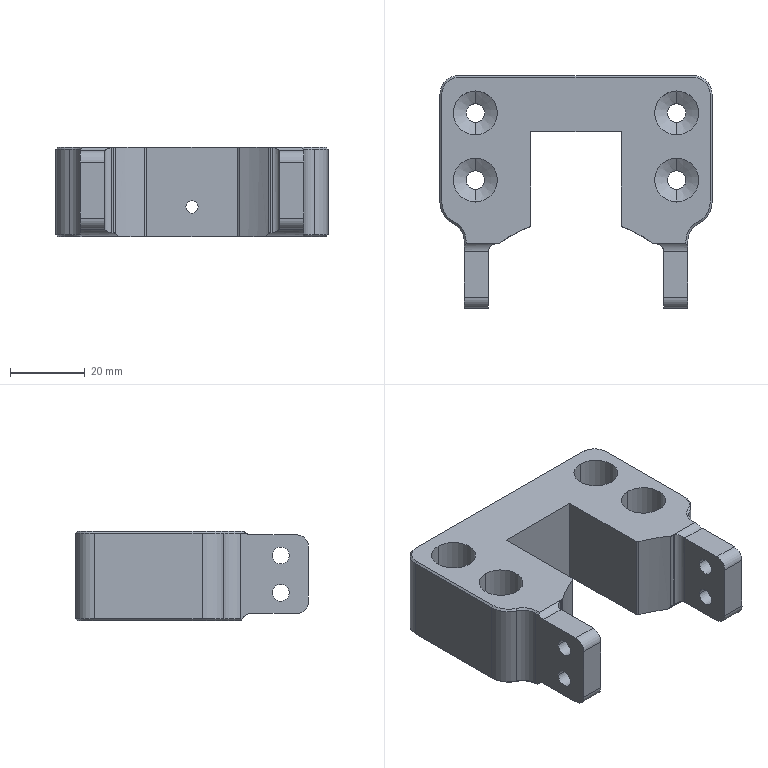NC program | NX | posted with a generic post | part box 73 x 62.4 x 24 mm
Lines 5456 to 6339 of 11507:
(ZLEVEL_PROFILE_COPY_1_COPY_1_COPY_1_1_COPY_COPY_COPY_1 , TOOL : D4)
N10832 T04 M6
N10834 G54
N10836 G17 G0 G90 X22.681 Y-16.85 S7000 M3
N10838 G43 Z30. H4
N10840 Z-0.231
N10842 G94 G1 X22.412 Y-16.271 F800.
N10844 G3 X22.084 Y-16.042 R0.4
N10846 G2 X21.5 Y-15.911 R2.236 F1500.
N10848 G1 X21.119
N10850 G2 X20.882 Y-15.901 R3.
N10852 G3 X20.521 Y-16.073 R0.4
N10854 G1 X20.166 Y-16.589
N10856 G0 X22.595 Y-17.112 Z-0.442
N10858 G1 X22.444 Y-16.527 F800.
N10860 G3 X22.165 Y-16.241 R0.4
N10862 G2 X21.5 Y-15.911 R1.977 F1500.
N10864 G1 X21.119
N10866 G2 X20.66 Y-15.875 R3.
N10868 G3 X20.287 Y-16.02 R0.4
N10870 G1 X19.894 Y-16.508
N10872 G0 X22.489 Y-17.386 Z-0.644
N10874 G1 X22.434 Y-16.785 F800.
N10876 G3 X22.203 Y-16.458 R0.4
N10878 G2 X21.5 Y-15.911 R1.965 F1500.
N10880 G1 X21.119
N10882 G2 X20.494 Y-15.845 R3.
N10884 G3 X20.113 Y-15.968 R0.4
N10886 G1 X19.694 Y-16.433
N10888 G0 X22.362 Y-17.646 Z-0.807
N10890 G1 X22.388 Y-17.042 F800.
N10892 G3 X22.203 Y-16.688 R0.4
N10894 G2 X21.5 Y-15.911 R1.975 F1500.
N10896 G1 X21.119
N10898 G2 X20.335 Y-15.806 R3.
N10900 G3 X19.948 Y-15.909 R0.4
N10902 G1 X19.504 Y-16.35
N10904 G0 X22.15 Y-17.871 Z-0.92
N10906 G1 X22.259 Y-17.277 F800.
N10908 G3 X22.124 Y-16.9 R0.4
N10910 G2 X21.5 Y-15.911 R1.961 F1500.
N10912 G1 X21.119
N10914 G2 X20.184 Y-15.761 R3.
N10916 G3 X19.793 Y-15.843 R0.4
N10918 G1 X19.326 Y-16.261
N10920 G0 X21.945 Y-18.069 Z-0.981
N10922 G1 X22.115 Y-17.491 F800.
N10924 G3 X22.021 Y-17.103 R0.4
N10926 G2 X21.5 Y-15.911 R1.903 F1500.
N10928 G1 X21.119
N10930 G2 X20.038 Y-15.709 R3.
N10932 G3 X19.643 Y-15.771 R0.4
N10934 G1 X19.155 Y-16.164
N10936 G0 X21.761 Y-18.168 Z-1.001
N10938 G1 X21.983 Y-17.59 F800.
N10940 G3 X21.921 Y-17.195 R0.4
N10942 G2 X21.5 Y-15.911 R1.897 F1500.
N10944 G1 X21.119
N10946 G2 X19.957 Y-15.676 R3.
N10948 G3 X19.561 Y-15.727 R0.4
N10950 G1 X19.062 Y-16.106
N10952 G0 X20.7 Y-19.155 Z-1.052
N10954 G1 X21.3 Y-18.808 F800.
N10956 G3 X21.5 Y-18.462 R0.4
N10958 G1 Y-15.911 F1500.
N10960 X21.119
N10962 G2 X19.585 Y-15.489 R3.
N10964 G3 X19.185 Y-15.483 R0.4
N10966 G1 X18.623 Y-15.798
N10968 G0 X20.7 Y-19.155 Z-1.155
N10970 G1 X21.3 Y-18.808 F800.
N10972 G3 X21.5 Y-18.462 R0.4
N10974 G1 Y-15.911 F1500.
N10976 X21.119
N10978 G2 X19.585 Y-15.489 R3.
N10980 G3 X19.185 Y-15.483 R0.4
N10982 G1 X18.623 Y-15.798
N10984 G0 X20.7 Y-19.155 Z-1.309
N10986 G1 X21.3 Y-18.808 F800.
N10988 G3 X21.5 Y-18.462 R0.4
N10990 G1 Y-15.911 F1500.
N10992 X21.119
N10994 G2 X19.585 Y-15.489 R3.
N10996 G3 X19.185 Y-15.483 R0.4
N10998 G1 X18.623 Y-15.798
N11000 G0 X20.7 Y-19.155 Z-1.51
N11002 G1 X21.3 Y-18.808 F800.
N11004 G3 X21.5 Y-18.462 R0.4
N11006 G1 Y-15.911 F1500.
N11008 X21.119
N11010 G2 X19.585 Y-15.489 R3.
N11012 G3 X19.185 Y-15.483 R0.4
N11014 G1 X18.623 Y-15.798
N11016 G0 X20.7 Y-19.155 Z-1.756
N11018 G1 X21.3 Y-18.808 F800.
N11020 G3 X21.5 Y-18.462 R0.4
N11022 G1 Y-15.911 F1500.
N11024 X21.119
N11026 G2 X19.585 Y-15.489 R3.
N11028 G3 X19.185 Y-15.483 R0.4
N11030 G1 X18.623 Y-15.798
N11032 G0 X20.7 Y-19.155 Z-2.041
N11034 G1 X21.3 Y-18.808 F800.
N11036 G3 X21.5 Y-18.462 R0.4
N11038 G1 Y-15.911 F1500.
N11040 X21.119
N11042 G2 X19.585 Y-15.489 R3.
N11044 G3 X19.185 Y-15.483 R0.4
N11046 G1 X18.623 Y-15.798
N11048 G0 X20.7 Y-19.155 Z-2.361
N11050 G1 X21.3 Y-18.808 F800.
N11052 G3 X21.5 Y-18.462 R0.4
N11054 G1 Y-15.911 F1500.
N11056 X21.119
N11058 G2 X19.585 Y-15.489 R3.
N11060 G3 X19.185 Y-15.483 R0.4
N11062 G1 X18.623 Y-15.798
N11064 G0 X20.7 Y-19.155 Z-2.71
N11066 G1 X21.3 Y-18.808 F800.
N11068 G3 X21.5 Y-18.462 R0.4
N11070 G1 Y-15.911 F1500.
N11072 X21.119
N11074 G2 X19.585 Y-15.489 R3.
N11076 G3 X19.185 Y-15.483 R0.4
N11078 G1 X18.623 Y-15.798
N11080 G0 X20.7 Y-19.155 Z-3.082
N11082 G1 X21.3 Y-18.808 F800.
N11084 G3 X21.5 Y-18.462 R0.4
N11086 G1 Y-15.911 F1500.
N11088 X21.119
N11090 G2 X19.585 Y-15.489 R3.
N11092 G3 X19.185 Y-15.483 R0.4
N11094 G1 X18.623 Y-15.798
N11096 G0 X20.7 Y-19.155 Z-3.47
N11098 G1 X21.3 Y-18.808 F800.
N11100 G3 X21.5 Y-18.462 R0.4
N11102 G1 Y-15.911 F1500.
N11104 X21.119
N11106 G2 X19.585 Y-15.489 R3.
N11108 G3 X19.185 Y-15.483 R0.4
N11110 G1 X18.623 Y-15.798
N11112 G0 X20.7 Y-19.155 Z-3.867
N11114 G1 X21.3 Y-18.808 F800.
N11116 G3 X21.5 Y-18.462 R0.4
N11118 G1 Y-15.911 F1500.
N11120 X21.119
N11122 G2 X19.585 Y-15.489 R3.
N11124 G3 X19.185 Y-15.483 R0.4
N11126 G1 X18.623 Y-15.798
N11128 G0 X20.7 Y-19.155 Z-4.267
N11130 G1 X21.3 Y-18.808 F800.
N11132 G3 X21.5 Y-18.462 R0.4
N11134 G1 Y-15.911 F1500.
N11136 X21.119
N11138 G2 X19.585 Y-15.489 R3.
N11140 G3 X19.185 Y-15.483 R0.4
N11142 G1 X18.623 Y-15.798
N11144 G0 X20.7 Y-19.155 Z-4.667
N11146 G1 X21.3 Y-18.808 F800.
N11148 G3 X21.5 Y-18.462 R0.4
N11150 G1 Y-15.911 F1500.
N11152 X21.119
N11154 G2 X19.585 Y-15.489 R3.
N11156 G3 X19.185 Y-15.483 R0.4
N11158 G1 X18.623 Y-15.798
N11160 G0 X20.7 Y-19.155 Z-5.067
N11162 G1 X21.3 Y-18.808 F800.
N11164 G3 X21.5 Y-18.462 R0.4
N11166 G1 Y-15.911 F1500.
N11168 X21.119
N11170 G2 X19.585 Y-15.489 R3.
N11172 G3 X19.185 Y-15.483 R0.4
N11174 G1 X18.623 Y-15.798
N11176 G0 X20.7 Y-19.155 Z-5.467
N11178 G1 X21.3 Y-18.808 F800.
N11180 G3 X21.5 Y-18.462 R0.4
N11182 G1 Y-15.911 F1500.
N11184 X21.119
N11186 G2 X19.585 Y-15.489 R3.
N11188 G3 X19.185 Y-15.483 R0.4
N11190 G1 X18.623 Y-15.798
N11192 G0 X20.7 Y-19.155 Z-5.867
N11194 G1 X21.3 Y-18.808 F800.
N11196 G3 X21.5 Y-18.462 R0.4
N11198 G1 Y-15.911 F1500.
N11200 X21.119
N11202 G2 X19.585 Y-15.489 R3.
N11204 G3 X19.185 Y-15.483 R0.4
N11206 G1 X18.623 Y-15.798
N11208 G0 X20.7 Y-19.155 Z-6.267
N11210 G1 X21.3 Y-18.808 F800.
N11212 G3 X21.5 Y-18.462 R0.4
N11214 G1 Y-15.911 F1500.
N11216 X21.119
N11218 G2 X19.585 Y-15.489 R3.
N11220 G3 X19.185 Y-15.483 R0.4
N11222 G1 X18.623 Y-15.798
N11224 G0 X20.7 Y-19.155 Z-6.667
N11226 G1 X21.3 Y-18.808 F800.
N11228 G3 X21.5 Y-18.462 R0.4
N11230 G1 Y-15.911 F1500.
N11232 X21.119
N11234 G2 X19.585 Y-15.489 R3.
N11236 G3 X19.185 Y-15.483 R0.4
N11238 G1 X18.623 Y-15.798
N11240 G0 X20.7 Y-19.155 Z-7.067
N11242 G1 X21.3 Y-18.808 F800.
N11244 G3 X21.5 Y-18.462 R0.4
N11246 G1 Y-15.911 F1500.
N11248 X21.119
N11250 G2 X19.585 Y-15.489 R3.
N11252 G3 X19.185 Y-15.483 R0.4
N11254 G1 X18.623 Y-15.798
N11256 G0 X20.7 Y-19.155 Z-7.467
N11258 G1 X21.3 Y-18.808 F800.
N11260 G3 X21.5 Y-18.462 R0.4
N11262 G1 Y-15.911 F1500.
N11264 X21.119
N11266 G2 X19.585 Y-15.489 R3.
N11268 G3 X19.185 Y-15.483 R0.4
N11270 G1 X18.623 Y-15.798
N11272 G0 X20.7 Y-19.155 Z-7.867
N11274 G1 X21.3 Y-18.808 F800.
N11276 G3 X21.5 Y-18.462 R0.4
N11278 G1 Y-15.911 F1500.
N11280 X21.119
N11282 G2 X19.585 Y-15.489 R3.
N11284 G3 X19.185 Y-15.483 R0.4
N11286 G1 X18.623 Y-15.798
N11288 G0 X20.7 Y-19.155 Z-8.267
N11290 G1 X21.3 Y-18.808 F800.
N11292 G3 X21.5 Y-18.462 R0.4
N11294 G1 Y-15.911 F1500.
N11296 X21.119
N11298 G2 X19.585 Y-15.489 R3.
N11300 G3 X19.185 Y-15.483 R0.4
N11302 G1 X18.623 Y-15.798
N11304 G0 X20.7 Y-19.155 Z-8.667
N11306 G1 X21.3 Y-18.808 F800.
N11308 G3 X21.5 Y-18.462 R0.4
N11310 G1 Y-15.911 F1500.
N11312 X21.119
N11314 G2 X19.585 Y-15.489 R3.
N11316 G3 X19.185 Y-15.483 R0.4
N11318 G1 X18.623 Y-15.798
N11320 G0 X20.7 Y-19.155 Z-9.067
N11322 G1 X21.3 Y-18.808 F800.
N11324 G3 X21.5 Y-18.462 R0.4
N11326 G1 Y-15.911 F1500.
N11328 X21.119
N11330 G2 X19.585 Y-15.489 R3.
N11332 G3 X19.185 Y-15.483 R0.4
N11334 G1 X18.623 Y-15.798
N11336 G0 X20.7 Y-19.155 Z-9.467
N11338 G1 X21.3 Y-18.808 F800.
N11340 G3 X21.5 Y-18.462 R0.4
N11342 G1 Y-15.911 F1500.
N11344 X21.119
N11346 G2 X19.585 Y-15.489 R3.
N11348 G3 X19.185 Y-15.483 R0.4
N11350 G1 X18.623 Y-15.798
N11352 G0 X20.7 Y-19.155 Z-9.867
N11354 G1 X21.3 Y-18.808 F800.
N11356 G3 X21.5 Y-18.462 R0.4
N11358 G1 Y-15.911 F1500.
N11360 X21.119
N11362 G2 X19.585 Y-15.489 R3.
N11364 G3 X19.185 Y-15.483 R0.4
N11366 G1 X18.623 Y-15.798
N11368 G0 X20.7 Y-19.155 Z-10.267
N11370 G1 X21.3 Y-18.808 F800.
N11372 G3 X21.5 Y-18.462 R0.4
N11374 G1 Y-15.911 F1500.
N11376 X21.119
N11378 G2 X19.585 Y-15.489 R3.
N11380 G3 X19.185 Y-15.483 R0.4
N11382 G1 X18.623 Y-15.798
N11384 G0 X20.7 Y-19.155 Z-10.667
N11386 G1 X21.3 Y-18.808 F800.
N11388 G3 X21.5 Y-18.462 R0.4
N11390 G1 Y-15.911 F1500.
N11392 X21.119
N11394 G2 X19.585 Y-15.489 R3.
N11396 G3 X19.185 Y-15.483 R0.4
N11398 G1 X18.623 Y-15.798
N11400 G0 X20.7 Y-19.155 Z-11.067
N11402 G1 X21.3 Y-18.808 F800.
N11404 G3 X21.5 Y-18.462 R0.4
N11406 G1 Y-15.911 F1500.
N11408 X21.119
N11410 G2 X19.585 Y-15.489 R3.
N11412 G3 X19.185 Y-15.483 R0.4
N11414 G1 X18.623 Y-15.798
N11416 G0 X20.7 Y-19.155 Z-11.467
N11418 G1 X21.3 Y-18.808 F800.
N11420 G3 X21.5 Y-18.462 R0.4
N11422 G1 Y-15.911 F1500.
N11424 X21.119
N11426 G2 X19.585 Y-15.489 R3.
N11428 G3 X19.185 Y-15.483 R0.4
N11430 G1 X18.623 Y-15.798
N11432 G0 X20.7 Y-19.155 Z-11.867
N11434 G1 X21.3 Y-18.808 F800.
N11436 G3 X21.5 Y-18.462 R0.4
N11438 G1 Y-15.911 F1500.
N11440 X21.119
N11442 G2 X19.585 Y-15.489 R3.
N11444 G3 X19.185 Y-15.483 R0.4
N11446 G1 X18.623 Y-15.798
N11448 G0 X20.7 Y-19.155 Z-12.267
N11450 G1 X21.3 Y-18.808 F800.
N11452 G3 X21.5 Y-18.462 R0.4
N11454 G1 Y-15.911 F1500.
N11456 X21.119
N11458 G2 X19.585 Y-15.489 R3.
N11460 G3 X19.185 Y-15.483 R0.4
N11462 G1 X18.623 Y-15.798
N11464 G0 X20.7 Y-19.155 Z-12.667
N11466 G1 X21.3 Y-18.808 F800.
N11468 G3 X21.5 Y-18.462 R0.4
N11470 G1 Y-15.911 F1500.
N11472 X21.119
N11474 G2 X19.585 Y-15.489 R3.
N11476 G3 X19.185 Y-15.483 R0.4
N11478 G1 X18.623 Y-15.798
N11480 G0 X20.7 Y-19.155 Z-13.067
N11482 G1 X21.3 Y-18.808 F800.
N11484 G3 X21.5 Y-18.462 R0.4
N11486 G1 Y-15.911 F1500.
N11488 X21.119
N11490 G2 X19.585 Y-15.489 R3.
N11492 G3 X19.185 Y-15.483 R0.4
N11494 G1 X18.623 Y-15.798
N11496 G0 X20.7 Y-19.155 Z-13.467
N11498 G1 X21.3 Y-18.808 F800.
N11500 G3 X21.5 Y-18.462 R0.4
N11502 G1 Y-15.911 F1500.
N11504 X21.119
N11506 G2 X19.585 Y-15.489 R3.
N11508 G3 X19.185 Y-15.483 R0.4
N11510 G1 X18.623 Y-15.798
N11512 G0 X20.7 Y-19.155 Z-13.867
N11514 G1 X21.3 Y-18.808 F800.
N11516 G3 X21.5 Y-18.462 R0.4
N11518 G1 Y-15.911 F1500.
N11520 X21.119
N11522 G2 X19.585 Y-15.489 R3.
N11524 G3 X19.185 Y-15.483 R0.4
N11526 G1 X18.623 Y-15.798
N11528 G0 X20.7 Y-19.155 Z-14.267
N11530 G1 X21.3 Y-18.808 F800.
N11532 G3 X21.5 Y-18.462 R0.4
N11534 G1 Y-15.911 F1500.
N11536 X21.119
N11538 G2 X19.585 Y-15.489 R3.
N11540 G3 X19.185 Y-15.483 R0.4
N11542 G1 X18.623 Y-15.798
N11544 G0 X20.7 Y-19.155 Z-14.667
N11546 G1 X21.3 Y-18.808 F800.
N11548 G3 X21.5 Y-18.462 R0.4
N11550 G1 Y-15.911 F1500.
N11552 X21.119
N11554 G2 X19.585 Y-15.489 R3.
N11556 G3 X19.185 Y-15.483 R0.4
N11558 G1 X18.623 Y-15.798
N11560 G0 X20.7 Y-19.155 Z-15.067
N11562 G1 X21.3 Y-18.808 F800.
N11564 G3 X21.5 Y-18.462 R0.4
N11566 G1 Y-15.911 F1500.
N11568 X21.119
N11570 G2 X19.585 Y-15.489 R3.
N11572 G3 X19.185 Y-15.483 R0.4
N11574 G1 X18.623 Y-15.798
N11576 G0 X20.7 Y-19.155 Z-15.467
N11578 G1 X21.3 Y-18.808 F800.
N11580 G3 X21.5 Y-18.462 R0.4
N11582 G1 Y-15.911 F1500.
N11584 X21.119
N11586 G2 X19.585 Y-15.489 R3.
N11588 G3 X19.185 Y-15.483 R0.4
N11590 G1 X18.623 Y-15.798
N11592 G0 X20.7 Y-19.155 Z-15.867
N11594 G1 X21.3 Y-18.808 F800.
N11596 G3 X21.5 Y-18.462 R0.4
N11598 G1 Y-15.911 F1500.
N11600 X21.119
N11602 G2 X19.585 Y-15.489 R3.
N11604 G3 X19.185 Y-15.483 R0.4
N11606 G1 X18.623 Y-15.798
N11608 G0 X20.7 Y-19.155 Z-16.267
N11610 G1 X21.3 Y-18.808 F800.
N11612 G3 X21.5 Y-18.462 R0.4
N11614 G1 Y-15.911 F1500.
N11616 X21.119
N11618 G2 X19.585 Y-15.489 R3.
N11620 G3 X19.185 Y-15.483 R0.4
N11622 G1 X18.623 Y-15.798
N11624 G0 X20.7 Y-19.155 Z-16.667
N11626 G1 X21.3 Y-18.808 F800.
N11628 G3 X21.5 Y-18.462 R0.4
N11630 G1 Y-15.911 F1500.
N11632 X21.119
N11634 G2 X19.585 Y-15.489 R3.
N11636 G3 X19.185 Y-15.483 R0.4
N11638 G1 X18.623 Y-15.798
N11640 G0 X20.7 Y-19.155 Z-17.067
N11642 G1 X21.3 Y-18.808 F800.
N11644 G3 X21.5 Y-18.462 R0.4
N11646 G1 Y-15.911 F1500.
N11648 X21.119
N11650 G2 X19.585 Y-15.489 R3.
N11652 G3 X19.185 Y-15.483 R0.4
N11654 G1 X18.623 Y-15.798
N11656 G0 X20.7 Y-19.155 Z-17.467
N11658 G1 X21.3 Y-18.808 F800.
N11660 G3 X21.5 Y-18.462 R0.4
N11662 G1 Y-15.911 F1500.
N11664 X21.119
N11666 G2 X19.585 Y-15.489 R3.
N11668 G3 X19.185 Y-15.483 R0.4
N11670 G1 X18.623 Y-15.798
N11672 G0 X20.7 Y-19.155 Z-17.867
N11674 G1 X21.3 Y-18.808 F800.
N11676 G3 X21.5 Y-18.462 R0.4
N11678 G1 Y-15.911 F1500.
N11680 X21.119
N11682 G2 X19.585 Y-15.489 R3.
N11684 G3 X19.185 Y-15.483 R0.4
N11686 G1 X18.623 Y-15.798
N11688 G0 X20.7 Y-19.155 Z-18.267
N11690 G1 X21.3 Y-18.808 F800.
N11692 G3 X21.5 Y-18.462 R0.4
N11694 G1 Y-15.911 F1500.
N11696 X21.119
N11698 G2 X19.585 Y-15.489 R3.
N11700 G3 X19.185 Y-15.483 R0.4
N11702 G1 X18.623 Y-15.798
N11704 G0 X20.7 Y-19.155 Z-18.667
N11706 G1 X21.3 Y-18.808 F800.
N11708 G3 X21.5 Y-18.462 R0.4
N11710 G1 Y-15.911 F1500.
N11712 X21.119
N11714 G2 X19.585 Y-15.489 R3.
N11716 G3 X19.185 Y-15.483 R0.4
N11718 G1 X18.623 Y-15.798
N11720 G0 X20.7 Y-19.155 Z-19.067
N11722 G1 X21.3 Y-18.808 F800.
N11724 G3 X21.5 Y-18.462 R0.4
N11726 G1 Y-15.911 F1500.
N11728 X21.119
N11730 G2 X19.585 Y-15.489 R3.
N11732 G3 X19.185 Y-15.483 R0.4
N11734 G1 X18.623 Y-15.798
N11736 G0 X20.7 Y-19.155 Z-19.467
N11738 G1 X21.3 Y-18.808 F800.
N11740 G3 X21.5 Y-18.462 R0.4
N11742 G1 Y-15.911 F1500.
N11744 X21.119
N11746 G2 X19.585 Y-15.489 R3.
N11748 G3 X19.185 Y-15.483 R0.4
N11750 G1 X18.623 Y-15.798
N11752 G0 X20.7 Y-19.155 Z-19.867
N11754 G1 X21.3 Y-18.808 F800.
N11756 G3 X21.5 Y-18.462 R0.4
N11758 G1 Y-15.911 F1500.
N11760 X21.119
N11762 G2 X19.585 Y-15.489 R3.
N11764 G3 X19.185 Y-15.483 R0.4
N11766 G1 X18.623 Y-15.798
N11768 G0 X20.7 Y-19.155 Z-20.267
N11770 G1 X21.3 Y-18.808 F800.
N11772 G3 X21.5 Y-18.462 R0.4
N11774 G1 Y-15.911 F1500.
N11776 X21.119
N11778 G2 X19.585 Y-15.489 R3.
N11780 G3 X19.185 Y-15.483 R0.4
N11782 G1 X18.623 Y-15.798
N11784 G0 X20.7 Y-19.155 Z-20.667
N11786 G1 X21.3 Y-18.808 F800.
N11788 G3 X21.5 Y-18.462 R0.4
N11790 G1 Y-15.911 F1500.
N11792 X21.119
N11794 G2 X19.585 Y-15.489 R3.
N11796 G3 X19.185 Y-15.483 R0.4
N11798 G1 X18.623 Y-15.798
N11800 G0 X20.7 Y-19.155 Z-21.067
N11802 G1 X21.3 Y-18.808 F800.
N11804 G3 X21.5 Y-18.462 R0.4
N11806 G1 Y-15.911 F1500.
N11808 X21.119
N11810 G2 X19.585 Y-15.489 R3.
N11812 G3 X19.185 Y-15.483 R0.4
N11814 G1 X18.623 Y-15.798
N11816 G0 X20.7 Y-19.155 Z-21.467
N11818 G1 X21.3 Y-18.808 F800.
N11820 G3 X21.5 Y-18.462 R0.4
N11822 G1 Y-15.911 F1500.
N11824 X21.119
N11826 G2 X19.585 Y-15.489 R3.
N11828 G3 X19.185 Y-15.483 R0.4
N11830 G1 X18.623 Y-15.798
N11832 G0 X20.7 Y-19.155 Z-21.867
N11834 G1 X21.3 Y-18.808 F800.
N11836 G3 X21.5 Y-18.462 R0.4
N11838 G1 Y-15.911 F1500.
N11840 X21.119
N11842 G2 X19.585 Y-15.489 R3.
N11844 G3 X19.185 Y-15.483 R0.4
N11846 G1 X18.623 Y-15.798
N11848 G0 X20.7 Y-19.155 Z-22.267
N11850 G1 X21.3 Y-18.808 F800.
N11852 G3 X21.5 Y-18.462 R0.4
N11854 G1 Y-15.911 F1500.
N11856 X21.119
N11858 G2 X19.585 Y-15.489 R3.
N11860 G3 X19.185 Y-15.483 R0.4
N11862 G1 X18.623 Y-15.798
N11864 G0 X20.7 Y-19.155 Z-22.667
N11866 G1 X21.3 Y-18.808 F800.
N11868 G3 X21.5 Y-18.462 R0.4
N11870 G1 Y-15.911 F1500.
N11872 X21.119
N11874 G2 X19.585 Y-15.489 R3.
N11876 G3 X19.185 Y-15.483 R0.4
N11878 G1 X18.623 Y-15.798
N11880 G0 X20.7 Y-19.155 Z-23.
N11882 G1 X21.3 Y-18.808 F800.
N11884 G3 X21.5 Y-18.462 R0.4
N11886 G1 Y-15.911 F1500.
N11888 X21.119
N11890 G2 X19.585 Y-15.489 R3.
N11892 G3 X19.185 Y-15.483 R0.4
N11894 G1 X18.623 Y-15.798
N11896 G0 X20.7 Y-19.141 Z-23.334
N11898 G1 X21.3 Y-18.795 F800.
N11900 G3 X21.5 Y-18.449 R0.4
N11902 G1 Y-15.911 F1500.
N11904 X21.119
N11906 G2 X19.599 Y-15.497 R3.
N11908 G3 X19.199 Y-15.494 R0.4
N11910 G1 X18.641 Y-15.81
N11912 G0 X20.7 Y-19.141 Z-23.667
N11914 G1 X21.3 Y-18.795 F800.
N11916 G3 X21.5 Y-18.449 R0.4
N11918 G1 Y-15.911 F1500.
N11920 X21.119
N11922 G2 X19.599 Y-15.497 R3.
N11924 G3 X19.199 Y-15.494 R0.4
N11926 G1 X18.641 Y-15.81
N11928 G0 X20.7 Y-19.141 Z-24.
N11930 G1 X21.3 Y-18.795 F800.
N11932 G3 X21.5 Y-18.449 R0.4
N11934 G1 Y-15.911 F1500.
N11936 X21.119
N11938 G2 X19.599 Y-15.497 R3.
N11940 G3 X19.199 Y-15.494 R0.4
N11942 G1 X18.641 Y-15.81
N11944 G0 Z30.
N11946 X9.3 Y10.354
N11948 Z-0.231
N11950 G1 X9.9 Y10.701 F800.
N11952 G3 X10.1 Y11.047 R0.4
N11954 G1 Y14.2 F1500.
N11956 X6.947
N11958 G3 X6.601 Y14. R0.4
N11960 G1 X6.254 Y13.4
N11962 G0 X9.3 Y10.354 Z-0.442
N11964 G1 X9.9 Y10.701 F800.
N11966 G3 X10.1 Y11.047 R0.4
N11968 G1 Y14.2 F1500.
N11970 X6.947
N11972 G3 X6.601 Y14. R0.4
N11974 G1 X6.254 Y13.4
N11976 G0 X9.3 Y10.354 Z-0.644
N11978 G1 X9.9 Y10.701 F800.
N11980 G3 X10.1 Y11.047 R0.4
N11982 G1 Y14.2 F1500.
N11984 X6.947
N11986 G3 X6.601 Y14. R0.4
N11988 G1 X6.254 Y13.4
N11990 G0 X9.3 Y10.354 Z-0.807
N11992 G1 X9.9 Y10.701 F800.
N11994 G3 X10.1 Y11.047 R0.4
N11996 G1 Y14.2 F1500.
N11998 X6.947
N12000 G3 X6.601 Y14. R0.4
N12002 G1 X6.254 Y13.4
N12004 G0 X9.3 Y10.354 Z-0.92
N12006 G1 X9.9 Y10.701 F800.
N12008 G3 X10.1 Y11.047 R0.4
N12010 G1 Y14.2 F1500.
N12012 X6.947
N12014 G3 X6.601 Y14. R0.4
N12016 G1 X6.254 Y13.4
N12018 G0 X9.3 Y10.354 Z-0.981
N12020 G1 X9.9 Y10.701 F800.
N12022 G3 X10.1 Y11.047 R0.4
N12024 G1 Y14.2 F1500.
N12026 X6.947
N12028 G3 X6.601 Y14. R0.4
N12030 G1 X6.254 Y13.4
N12032 G0 X9.3 Y10.354 Z-1.001
N12034 G1 X9.9 Y10.701 F800.
N12036 G3 X10.1 Y11.047 R0.4
N12038 G1 Y14.2 F1500.
N12040 X6.947
N12042 G3 X6.601 Y14. R0.4
N12044 G1 X6.254 Y13.4
N12046 G0 X9.3 Y10.354 Z-1.052
N12048 G1 X9.9 Y10.701 F800.
N12050 G3 X10.1 Y11.047 R0.4
N12052 G1 Y14.2 F1500.
N12054 X6.947
N12056 G3 X6.601 Y14. R0.4
N12058 G1 X6.254 Y13.4
N12060 G0 X9.3 Y10.354 Z-1.155
N12062 G1 X9.9 Y10.701 F800.
N12064 G3 X10.1 Y11.047 R0.4
N12066 G1 Y14.2 F1500.
N12068 X6.947
N12070 G3 X6.601 Y14. R0.4
N12072 G1 X6.254 Y13.4
N12074 G0 X9.3 Y10.354 Z-1.309
N12076 G1 X9.9 Y10.701 F800.
N12078 G3 X10.1 Y11.047 R0.4
N12080 G1 Y14.2 F1500.
N12082 X6.947
N12084 G3 X6.601 Y14. R0.4
N12086 G1 X6.254 Y13.4
N12088 G0 X9.3 Y10.354 Z-1.51
N12090 G1 X9.9 Y10.701 F800.
N12092 G3 X10.1 Y11.047 R0.4
N12094 G1 Y14.2 F1500.
N12096 X6.947
N12098 G3 X6.601 Y14. R0.4
N12100 G1 X6.254 Y13.4
N12102 G0 X9.3 Y10.354 Z-1.756
N12104 G1 X9.9 Y10.701 F800.
N12106 G3 X10.1 Y11.047 R0.4
N12108 G1 Y14.2 F1500.
N12110 X6.947
N12112 G3 X6.601 Y14. R0.4
N12114 G1 X6.254 Y13.4
N12116 G0 X9.3 Y10.354 Z-2.041
N12118 G1 X9.9 Y10.701 F800.
N12120 G3 X10.1 Y11.047 R0.4
N12122 G1 Y14.2 F1500.
N12124 X6.947
N12126 G3 X6.601 Y14. R0.4
N12128 G1 X6.254 Y13.4
N12130 G0 X9.3 Y10.354 Z-2.361
N12132 G1 X9.9 Y10.701 F800.
N12134 G3 X10.1 Y11.047 R0.4
N12136 G1 Y14.2 F1500.
N12138 X6.947
N12140 G3 X6.601 Y14. R0.4
N12142 G1 X6.254 Y13.4
N12144 G0 X9.3 Y10.354 Z-2.71
N12146 G1 X9.9 Y10.701 F800.
N12148 G3 X10.1 Y11.047 R0.4
N12150 G1 Y14.2 F1500.
N12152 X6.947
N12154 G3 X6.601 Y14. R0.4
N12156 G1 X6.254 Y13.4
N12158 G0 X9.3 Y10.354 Z-3.082
N12160 G1 X9.9 Y10.701 F800.
N12162 G3 X10.1 Y11.047 R0.4
N12164 G1 Y14.2 F1500.
N12166 X6.947
N12168 G3 X6.601 Y14. R0.4
N12170 G1 X6.254 Y13.4
N12172 G0 X9.3 Y10.354 Z-3.47
N12174 G1 X9.9 Y10.701 F800.
N12176 G3 X10.1 Y11.047 R0.4
N12178 G1 Y14.2 F1500.
N12180 X6.947
N12182 G3 X6.601 Y14. R0.4
N12184 G1 X6.254 Y13.4
N12186 G0 X9.3 Y10.354 Z-3.867
N12188 G1 X9.9 Y10.701 F800.
N12190 G3 X10.1 Y11.047 R0.4
N12192 G1 Y14.2 F1500.
N12194 X6.947
N12196 G3 X6.601 Y14. R0.4
N12198 G1 X6.254 Y13.4
N12200 G0 X9.3 Y10.354 Z-4.267
N12202 G1 X9.9 Y10.701 F800.
N12204 G3 X10.1 Y11.047 R0.4
N12206 G1 Y14.2 F1500.
N12208 X6.947
N12210 G3 X6.601 Y14. R0.4
N12212 G1 X6.254 Y13.4
N12214 G0 X9.3 Y10.354 Z-4.667
N12216 G1 X9.9 Y10.701 F800.
N12218 G3 X10.1 Y11.047 R0.4
N12220 G1 Y14.2 F1500.
N12222 X6.947
N12224 G3 X6.601 Y14. R0.4
N12226 G1 X6.254 Y13.4
N12228 G0 X9.3 Y10.354 Z-5.067
N12230 G1 X9.9 Y10.701 F800.
N12232 G3 X10.1 Y11.047 R0.4
N12234 G1 Y14.2 F1500.
N12236 X6.947
N12238 G3 X6.601 Y14. R0.4
N12240 G1 X6.254 Y13.4
N12242 G0 X9.3 Y10.354 Z-5.467
N12244 G1 X9.9 Y10.701 F800.
N12246 G3 X10.1 Y11.047 R0.4
N12248 G1 Y14.2 F1500.
N12250 X6.947
N12252 G3 X6.601 Y14. R0.4
N12254 G1 X6.254 Y13.4
N12256 G0 X9.3 Y10.354 Z-5.867
N12258 G1 X9.9 Y10.701 F800.
N12260 G3 X10.1 Y11.047 R0.4
N12262 G1 Y14.2 F1500.
N12264 X6.947
N12266 G3 X6.601 Y14. R0.4
N12268 G1 X6.254 Y13.4
N12270 G0 X9.3 Y10.354 Z-6.267
N12272 G1 X9.9 Y10.701 F800.
N12274 G3 X10.1 Y11.047 R0.4
N12276 G1 Y14.2 F1500.
N12278 X6.947
N12280 G3 X6.601 Y14. R0.4
N12282 G1 X6.254 Y13.4
N12284 G0 X9.3 Y10.354 Z-6.667
N12286 G1 X9.9 Y10.701 F800.
N12288 G3 X10.1 Y11.047 R0.4
N12290 G1 Y14.2 F1500.
N12292 X6.947
N12294 G3 X6.601 Y14. R0.4
N12296 G1 X6.254 Y13.4
N12298 G0 X9.3 Y10.354 Z-7.067
N12300 G1 X9.9 Y10.701 F800.
N12302 G3 X10.1 Y11.047 R0.4
N12304 G1 Y14.2 F1500.
N12306 X6.947
N12308 G3 X6.601 Y14. R0.4
N12310 G1 X6.254 Y13.4
N12312 G0 X9.3 Y10.354 Z-7.467
N12314 G1 X9.9 Y10.701 F800.
N12316 G3 X10.1 Y11.047 R0.4
N12318 G1 Y14.2 F1500.
N12320 X6.947
N12322 G3 X6.601 Y14. R0.4
N12324 G1 X6.254 Y13.4
N12326 G0 X9.3 Y10.354 Z-7.867
N12328 G1 X9.9 Y10.701 F800.
N12330 G3 X10.1 Y11.047 R0.4
N12332 G1 Y14.2 F1500.
N12334 X6.947
N12336 G3 X6.601 Y14. R0.4
N12338 G1 X6.254 Y13.4
N12340 G0 X9.3 Y10.354 Z-8.267
N12342 G1 X9.9 Y10.701 F800.
N12344 G3 X10.1 Y11.047 R0.4
N12346 G1 Y14.2 F1500.
N12348 X6.947
N12350 G3 X6.601 Y14. R0.4
N12352 G1 X6.254 Y13.4
N12354 G0 X9.3 Y10.354 Z-8.667
N12356 G1 X9.9 Y10.701 F800.
N12358 G3 X10.1 Y11.047 R0.4
N12360 G1 Y14.2 F1500.
N12362 X6.947
N12364 G3 X6.601 Y14. R0.4
N12366 G1 X6.254 Y13.4
N12368 G0 X9.3 Y10.354 Z-9.067
N12370 G1 X9.9 Y10.701 F800.
N12372 G3 X10.1 Y11.047 R0.4
N12374 G1 Y14.2 F1500.
N12376 X6.947
N12378 G3 X6.601 Y14. R0.4
N12380 G1 X6.254 Y13.4
N12382 G0 X9.3 Y10.354 Z-9.467
N12384 G1 X9.9 Y10.701 F800.
N12386 G3 X10.1 Y11.047 R0.4
N12388 G1 Y14.2 F1500.
N12390 X6.947
N12392 G3 X6.601 Y14. R0.4
N12394 G1 X6.254 Y13.4
N12396 G0 X9.3 Y10.354 Z-9.867
N12398 G1 X9.9 Y10.701 F800.
N12400 G3 X10.1 Y11.047 R0.4
N12402 G1 Y14.2 F1500.
N12404 X6.947
N12406 G3 X6.601 Y14. R0.4
N12408 G1 X6.254 Y13.4
N12410 G0 X9.3 Y10.354 Z-10.267
N12412 G1 X9.9 Y10.701 F800.
N12414 G3 X10.1 Y11.047 R0.4
N12416 G1 Y14.2 F1500.
N12418 X6.947
N12420 G3 X6.601 Y14. R0.4
N12422 G1 X6.254 Y13.4
N12424 G0 X9.3 Y10.354 Z-10.667
N12426 G1 X9.9 Y10.701 F800.
N12428 G3 X10.1 Y11.047 R0.4
N12430 G1 Y14.2 F1500.
N12432 X6.947
N12434 G3 X6.601 Y14. R0.4
N12436 G1 X6.254 Y13.4
N12438 G0 X9.3 Y10.354 Z-11.067
N12440 G1 X9.9 Y10.701 F800.
N12442 G3 X10.1 Y11.047 R0.4
N12444 G1 Y14.2 F1500.
N12446 X6.947
N12448 G3 X6.601 Y14. R0.4
N12450 G1 X6.254 Y13.4
N12452 G0 X9.3 Y10.354 Z-11.467
N12454 G1 X9.9 Y10.701 F800.
N12456 G3 X10.1 Y11.047 R0.4
N12458 G1 Y14.2 F1500.
N12460 X6.947
N12462 G3 X6.601 Y14. R0.4
N12464 G1 X6.254 Y13.4
N12466 G0 X9.3 Y10.354 Z-11.867
N12468 G1 X9.9 Y10.701 F800.
N12470 G3 X10.1 Y11.047 R0.4
N12472 G1 Y14.2 F1500.
N12474 X6.947
N12476 G3 X6.601 Y14. R0.4
N12478 G1 X6.254 Y13.4
N12480 G0 X9.3 Y10.354 Z-12.267
N12482 G1 X9.9 Y10.701 F800.
N12484 G3 X10.1 Y11.047 R0.4
N12486 G1 Y14.2 F1500.
N12488 X6.947
N12490 G3 X6.601 Y14. R0.4
N12492 G1 X6.254 Y13.4
N12494 G0 X9.3 Y10.354 Z-12.667
N12496 G1 X9.9 Y10.701 F800.
N12498 G3 X10.1 Y11.047 R0.4
N12500 G1 Y14.2 F1500.
N12502 X6.947
N12504 G3 X6.601 Y14. R0.4
N12506 G1 X6.254 Y13.4
N12508 G0 X9.3 Y10.354 Z-13.067
N12510 G1 X9.9 Y10.701 F800.
N12512 G3 X10.1 Y11.047 R0.4
N12514 G1 Y14.2 F1500.
N12516 X6.947
N12518 G3 X6.601 Y14. R0.4
N12520 G1 X6.254 Y13.4
N12522 G0 X9.3 Y10.354 Z-13.467
N12524 G1 X9.9 Y10.701 F800.
N12526 G3 X10.1 Y11.047 R0.4
N12528 G1 Y14.2 F1500.
N12530 X6.947
N12532 G3 X6.601 Y14. R0.4
N12534 G1 X6.254 Y13.4
N12536 G0 X9.3 Y10.354 Z-13.867
N12538 G1 X9.9 Y10.701 F800.
N12540 G3 X10.1 Y11.047 R0.4
N12542 G1 Y14.2 F1500.
N12544 X6.947
N12546 G3 X6.601 Y14. R0.4
N12548 G1 X6.254 Y13.4
N12550 G0 X9.3 Y10.354 Z-14.267
N12552 G1 X9.9 Y10.701 F800.
N12554 G3 X10.1 Y11.047 R0.4
N12556 G1 Y14.2 F1500.
N12558 X6.947
N12560 G3 X6.601 Y14. R0.4
N12562 G1 X6.254 Y13.4
N12564 G0 X9.3 Y10.354 Z-14.667
N12566 G1 X9.9 Y10.701 F800.
N12568 G3 X10.1 Y11.047 R0.4
N12570 G1 Y14.2 F1500.
N12572 X6.947
N12574 G3 X6.601 Y14. R0.4
N12576 G1 X6.254 Y13.4
N12578 G0 X9.3 Y10.354 Z-15.067
N12580 G1 X9.9 Y10.701 F800.
N12582 G3 X10.1 Y11.047 R0.4
N12584 G1 Y14.2 F1500.
N12586 X6.947
N12588 G3 X6.601 Y14. R0.4
N12590 G1 X6.254 Y13.4
N12592 G0 X9.3 Y10.354 Z-15.467